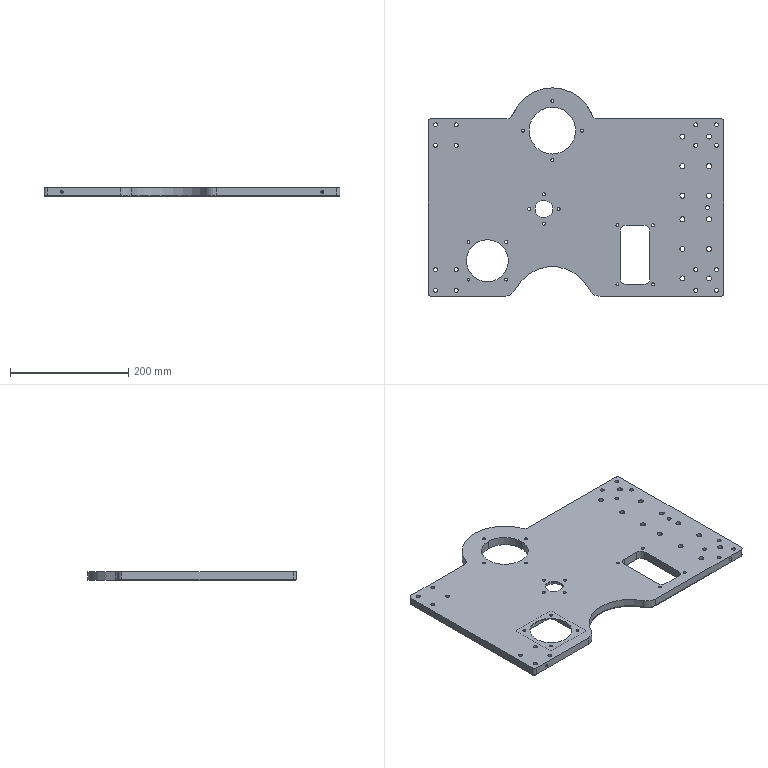NC program | Mastercam | posted with a generic post
Lines 4161 to 5460 of 11903, first 1119 of 1300 lines:
N1940 T6 M6
N1950 G0 G90 G17 G54 X237.5 Y-111.32 A0. S6000 M3
N1960 G43 H6 Z50. M8
N1970 Z1.3
N1980 G1 Z.3 F600.
N1990 G3 X235.07 Y-113.75 Z.175 I0. J-2.43 F3000.
N2000 X237.5 Y-116.18 Z.05 I2.43 J0.
N2010 X239.93 Y-113.75 Z-.075 I0. J2.43
N2020 X237.5 Y-111.32 Z-.2 I-2.43 J0.
N2030 X235.07 Y-113.75 Z-.325 I0. J-2.43
N2040 X237.5 Y-116.18 Z-.45 I2.43 J0.
N2050 X239.93 Y-113.75 Z-.575 I0. J2.43
N2060 X237.5 Y-111.32 Z-.7 I-2.43 J0.
N2070 X235.07 Y-113.75 Z-.825 I0. J-2.43
N2080 X237.5 Y-116.18 Z-.95 I2.43 J0.
N2090 X239.93 Y-113.75 Z-1.075 I0. J2.43
N2100 X237.5 Y-111.32 Z-1.2 I-2.43 J0.
N2110 X235.07 Y-113.75 Z-1.325 I0. J-2.43
N2120 X237.5 Y-116.18 Z-1.45 I2.43 J0.
N2130 X239.93 Y-113.75 Z-1.575 I0. J2.43
N2140 X237.5 Y-111.32 Z-1.7 I-2.43 J0.
N2150 X235.07 Y-113.75 Z-1.825 I0. J-2.43
N2160 X237.5 Y-116.18 Z-1.95 I2.43 J0.
N2170 X239.93 Y-113.75 Z-2.075 I0. J2.43
N2180 X237.5 Y-111.32 Z-2.2 I-2.43 J0.
N2190 X235.07 Y-113.75 Z-2.325 I0. J-2.43
N2200 X237.5 Y-116.18 Z-2.45 I2.43 J0.
N2210 X239.93 Y-113.75 Z-2.575 I0. J2.43
N2220 X237.5 Y-111.32 Z-2.7 I-2.43 J0.
N2230 X235.07 Y-113.75 Z-2.825 I0. J-2.43
N2240 X237.5 Y-116.18 Z-2.95 I2.43 J0.
N2250 X239.93 Y-113.75 Z-3.075 I0. J2.43
N2260 X237.5 Y-111.32 Z-3.2 I-2.43 J0.
N2270 X235.07 Y-113.75 Z-3.325 I0. J-2.43
N2280 X237.5 Y-116.18 Z-3.45 I2.43 J0.
N2290 X239.93 Y-113.75 Z-3.575 I0. J2.43
N2300 X237.5 Y-111.32 Z-3.7 I-2.43 J0.
N2310 X235.07 Y-113.75 Z-3.825 I0. J-2.43
N2320 X237.5 Y-116.18 Z-3.95 I2.43 J0.
N2330 X239.93 Y-113.75 Z-4.075 I0. J2.43
N2340 X237.5 Y-111.32 Z-4.2 I-2.43 J0.
N2350 X235.07 Y-113.75 Z-4.325 I0. J-2.43
N2360 X237.5 Y-116.18 Z-4.45 I2.43 J0.
N2370 X239.93 Y-113.75 Z-4.575 I0. J2.43
N2380 X237.5 Y-111.32 Z-4.7 I-2.43 J0.
N2390 X235.07 Y-113.75 Z-4.825 I0. J-2.43
N2400 X237.5 Y-116.18 Z-4.95 I2.43 J0.
N2410 X239.93 Y-113.75 Z-5.075 I0. J2.43
N2420 X237.5 Y-111.32 Z-5.2 I-2.43 J0.
N2430 X235.07 Y-113.75 Z-5.325 I0. J-2.43
N2440 X237.5 Y-116.18 Z-5.45 I2.43 J0.
N2450 X239.93 Y-113.75 Z-5.575 I0. J2.43
N2460 X237.5 Y-111.32 Z-5.7 I-2.43 J0.
N2470 X235.07 Y-113.75 Z-5.825 I0. J-2.43
N2480 X237.5 Y-116.18 Z-5.95 I2.43 J0.
N2490 X239.93 Y-113.75 Z-6.075 I0. J2.43
N2500 X237.5 Y-111.32 Z-6.2 I-2.43 J0.
N2510 X235.07 Y-113.75 Z-6.325 I0. J-2.43
N2520 X237.5 Y-116.18 Z-6.45 I2.43 J0.
N2530 X239.93 Y-113.75 Z-6.575 I0. J2.43
N2540 X237.5 Y-111.32 Z-6.7 I-2.43 J0.
N2550 X236.072 Y-111.784 Z-6.75 I0. J-2.43
N2560 X235.07 Y-113.75 I1.428 J-1.966
N2570 X237.5 Y-116.18 I2.43 J0.
N2580 X239.93 Y-113.75 I0. J2.43
N2590 X237.5 Y-111.32 I-2.43 J0.
N2600 X235.7 Y-112.117 I0. J-2.43
N2610 G0 Z50.
N2620 X202.5 Y-111.32
N2630 Z1.3
N2640 G1 Z.3 F600.
N2650 G3 X200.07 Y-113.75 Z.175 I0. J-2.43 F3000.
N2660 X202.5 Y-116.18 Z.05 I2.43 J0.
N2670 X204.93 Y-113.75 Z-.075 I0. J2.43
N2680 X202.5 Y-111.32 Z-.2 I-2.43 J0.
N2690 X200.07 Y-113.75 Z-.325 I0. J-2.43
N2700 X202.5 Y-116.18 Z-.45 I2.43 J0.
N2710 X204.93 Y-113.75 Z-.575 I0. J2.43
N2720 X202.5 Y-111.32 Z-.7 I-2.43 J0.
N2730 X200.07 Y-113.75 Z-.825 I0. J-2.43
N2740 X202.5 Y-116.18 Z-.95 I2.43 J0.
N2750 X204.93 Y-113.75 Z-1.075 I0. J2.43
N2760 X202.5 Y-111.32 Z-1.2 I-2.43 J0.
N2770 X200.07 Y-113.75 Z-1.325 I0. J-2.43
N2780 X202.5 Y-116.18 Z-1.45 I2.43 J0.
N2790 X204.93 Y-113.75 Z-1.575 I0. J2.43
N2800 X202.5 Y-111.32 Z-1.7 I-2.43 J0.
N2810 X200.07 Y-113.75 Z-1.825 I0. J-2.43
N2820 X202.5 Y-116.18 Z-1.95 I2.43 J0.
N2830 X204.93 Y-113.75 Z-2.075 I0. J2.43
N2840 X202.5 Y-111.32 Z-2.2 I-2.43 J0.
N2850 X200.07 Y-113.75 Z-2.325 I0. J-2.43
N2860 X202.5 Y-116.18 Z-2.45 I2.43 J0.
N2870 X204.93 Y-113.75 Z-2.575 I0. J2.43
N2880 X202.5 Y-111.32 Z-2.7 I-2.43 J0.
N2890 X200.07 Y-113.75 Z-2.825 I0. J-2.43
N2900 X202.5 Y-116.18 Z-2.95 I2.43 J0.
N2910 X204.93 Y-113.75 Z-3.075 I0. J2.43
N2920 X202.5 Y-111.32 Z-3.2 I-2.43 J0.
N2930 X200.07 Y-113.75 Z-3.325 I0. J-2.43
N2940 X202.5 Y-116.18 Z-3.45 I2.43 J0.
N2950 X204.93 Y-113.75 Z-3.575 I0. J2.43
N2960 X202.5 Y-111.32 Z-3.7 I-2.43 J0.
N2970 X200.07 Y-113.75 Z-3.825 I0. J-2.43
N2980 X202.5 Y-116.18 Z-3.95 I2.43 J0.
N2990 X204.93 Y-113.75 Z-4.075 I0. J2.43
N3000 X202.5 Y-111.32 Z-4.2 I-2.43 J0.
N3010 X200.07 Y-113.75 Z-4.325 I0. J-2.43
N3020 X202.5 Y-116.18 Z-4.45 I2.43 J0.
N3030 X204.93 Y-113.75 Z-4.575 I0. J2.43
N3040 X202.5 Y-111.32 Z-4.7 I-2.43 J0.
N3050 X200.07 Y-113.75 Z-4.825 I0. J-2.43
N3060 X202.5 Y-116.18 Z-4.95 I2.43 J0.
N3070 X204.93 Y-113.75 Z-5.075 I0. J2.43
N3080 X202.5 Y-111.32 Z-5.2 I-2.43 J0.
N3090 X200.07 Y-113.75 Z-5.325 I0. J-2.43
N3100 X202.5 Y-116.18 Z-5.45 I2.43 J0.
N3110 X204.93 Y-113.75 Z-5.575 I0. J2.43
N3120 X202.5 Y-111.32 Z-5.7 I-2.43 J0.
N3130 X200.07 Y-113.75 Z-5.825 I0. J-2.43
N3140 X202.5 Y-116.18 Z-5.95 I2.43 J0.
N3150 X204.93 Y-113.75 Z-6.075 I0. J2.43
N3160 X202.5 Y-111.32 Z-6.2 I-2.43 J0.
N3170 X200.07 Y-113.75 Z-6.325 I0. J-2.43
N3180 X202.5 Y-116.18 Z-6.45 I2.43 J0.
N3190 X204.93 Y-113.75 Z-6.575 I0. J2.43
N3200 X202.5 Y-111.32 Z-6.7 I-2.43 J0.
N3210 X201.072 Y-111.784 Z-6.75 I0. J-2.43
N3220 X200.07 Y-113.75 I1.428 J-1.966
N3230 X202.5 Y-116.18 I2.43 J0.
N3240 X204.93 Y-113.75 I0. J2.43
N3250 X202.5 Y-111.32 I-2.43 J0.
N3260 X200.7 Y-112.117 I0. J-2.43
N3270 G0 Z50.
N3280 X202.5 Y-76.32
N3290 Z1.3
N3300 G1 Z.3 F600.
N3310 G3 X200.07 Y-78.75 Z.175 I0. J-2.43 F3000.
N3320 X202.5 Y-81.18 Z.05 I2.43 J0.
N3330 X204.93 Y-78.75 Z-.075 I0. J2.43
N3340 X202.5 Y-76.32 Z-.2 I-2.43 J0.
N3350 X200.07 Y-78.75 Z-.325 I0. J-2.43
N3360 X202.5 Y-81.18 Z-.45 I2.43 J0.
N3370 X204.93 Y-78.75 Z-.575 I0. J2.43
N3380 X202.5 Y-76.32 Z-.7 I-2.43 J0.
N3390 X200.07 Y-78.75 Z-.825 I0. J-2.43
N3400 X202.5 Y-81.18 Z-.95 I2.43 J0.
N3410 X204.93 Y-78.75 Z-1.075 I0. J2.43
N3420 X202.5 Y-76.32 Z-1.2 I-2.43 J0.
N3430 X200.07 Y-78.75 Z-1.325 I0. J-2.43
N3440 X202.5 Y-81.18 Z-1.45 I2.43 J0.
N3450 X204.93 Y-78.75 Z-1.575 I0. J2.43
N3460 X202.5 Y-76.32 Z-1.7 I-2.43 J0.
N3470 X200.07 Y-78.75 Z-1.825 I0. J-2.43
N3480 X202.5 Y-81.18 Z-1.95 I2.43 J0.
N3490 X204.93 Y-78.75 Z-2.075 I0. J2.43
N3500 X202.5 Y-76.32 Z-2.2 I-2.43 J0.
N3510 X200.07 Y-78.75 Z-2.325 I0. J-2.43
N3520 X202.5 Y-81.18 Z-2.45 I2.43 J0.
N3530 X204.93 Y-78.75 Z-2.575 I0. J2.43
N3540 X202.5 Y-76.32 Z-2.7 I-2.43 J0.
N3550 X200.07 Y-78.75 Z-2.825 I0. J-2.43
N3560 X202.5 Y-81.18 Z-2.95 I2.43 J0.
N3570 X204.93 Y-78.75 Z-3.075 I0. J2.43
N3580 X202.5 Y-76.32 Z-3.2 I-2.43 J0.
N3590 X200.07 Y-78.75 Z-3.325 I0. J-2.43
N3600 X202.5 Y-81.18 Z-3.45 I2.43 J0.
N3610 X204.93 Y-78.75 Z-3.575 I0. J2.43
N3620 X202.5 Y-76.32 Z-3.7 I-2.43 J0.
N3630 X200.07 Y-78.75 Z-3.825 I0. J-2.43
N3640 X202.5 Y-81.18 Z-3.95 I2.43 J0.
N3650 X204.93 Y-78.75 Z-4.075 I0. J2.43
N3660 X202.5 Y-76.32 Z-4.2 I-2.43 J0.
N3670 X200.07 Y-78.75 Z-4.325 I0. J-2.43
N3680 X202.5 Y-81.18 Z-4.45 I2.43 J0.
N3690 X204.93 Y-78.75 Z-4.575 I0. J2.43
N3700 X202.5 Y-76.32 Z-4.7 I-2.43 J0.
N3710 X200.07 Y-78.75 Z-4.825 I0. J-2.43
N3720 X202.5 Y-81.18 Z-4.95 I2.43 J0.
N3730 X204.93 Y-78.75 Z-5.075 I0. J2.43
N3740 X202.5 Y-76.32 Z-5.2 I-2.43 J0.
N3750 X200.07 Y-78.75 Z-5.325 I0. J-2.43
N3760 X202.5 Y-81.18 Z-5.45 I2.43 J0.
N3770 X204.93 Y-78.75 Z-5.575 I0. J2.43
N3780 X202.5 Y-76.32 Z-5.7 I-2.43 J0.
N3790 X200.07 Y-78.75 Z-5.825 I0. J-2.43
N3800 X202.5 Y-81.18 Z-5.95 I2.43 J0.
N3810 X204.93 Y-78.75 Z-6.075 I0. J2.43
N3820 X202.5 Y-76.32 Z-6.2 I-2.43 J0.
N3830 X200.07 Y-78.75 Z-6.325 I0. J-2.43
N3840 X202.5 Y-81.18 Z-6.45 I2.43 J0.
N3850 X204.93 Y-78.75 Z-6.575 I0. J2.43
N3860 X202.5 Y-76.32 Z-6.7 I-2.43 J0.
N3870 X201.072 Y-76.784 Z-6.75 I0. J-2.43
N3880 X200.07 Y-78.75 I1.428 J-1.966
N3890 X202.5 Y-81.18 I2.43 J0.
N3900 X204.93 Y-78.75 I0. J2.43
N3910 X202.5 Y-76.32 I-2.43 J0.
N3920 X200.7 Y-77.117 I0. J-2.43
N3930 G0 Z50.
N3940 X237.5 Y-76.32
N3950 Z1.3
N3960 G1 Z.3 F600.
N3970 G3 X235.07 Y-78.75 Z.175 I0. J-2.43 F3000.
N3980 X237.5 Y-81.18 Z.05 I2.43 J0.
N3990 X239.93 Y-78.75 Z-.075 I0. J2.43
N4000 X237.5 Y-76.32 Z-.2 I-2.43 J0.
N4010 X235.07 Y-78.75 Z-.325 I0. J-2.43
N4020 X237.5 Y-81.18 Z-.45 I2.43 J0.
N4030 X239.93 Y-78.75 Z-.575 I0. J2.43
N4040 X237.5 Y-76.32 Z-.7 I-2.43 J0.
N4050 X235.07 Y-78.75 Z-.825 I0. J-2.43
N4060 X237.5 Y-81.18 Z-.95 I2.43 J0.
N4070 X239.93 Y-78.75 Z-1.075 I0. J2.43
N4080 X237.5 Y-76.32 Z-1.2 I-2.43 J0.
N4090 X235.07 Y-78.75 Z-1.325 I0. J-2.43
N4100 X237.5 Y-81.18 Z-1.45 I2.43 J0.
N4110 X239.93 Y-78.75 Z-1.575 I0. J2.43
N4120 X237.5 Y-76.32 Z-1.7 I-2.43 J0.
N4130 X235.07 Y-78.75 Z-1.825 I0. J-2.43
N4140 X237.5 Y-81.18 Z-1.95 I2.43 J0.
N4150 X239.93 Y-78.75 Z-2.075 I0. J2.43
N4160 X237.5 Y-76.32 Z-2.2 I-2.43 J0.
N4170 X235.07 Y-78.75 Z-2.325 I0. J-2.43
N4180 X237.5 Y-81.18 Z-2.45 I2.43 J0.
N4190 X239.93 Y-78.75 Z-2.575 I0. J2.43
N4200 X237.5 Y-76.32 Z-2.7 I-2.43 J0.
N4210 X235.07 Y-78.75 Z-2.825 I0. J-2.43
N4220 X237.5 Y-81.18 Z-2.95 I2.43 J0.
N4230 X239.93 Y-78.75 Z-3.075 I0. J2.43
N4240 X237.5 Y-76.32 Z-3.2 I-2.43 J0.
N4250 X235.07 Y-78.75 Z-3.325 I0. J-2.43
N4260 X237.5 Y-81.18 Z-3.45 I2.43 J0.
N4270 X239.93 Y-78.75 Z-3.575 I0. J2.43
N4280 X237.5 Y-76.32 Z-3.7 I-2.43 J0.
N4290 X235.07 Y-78.75 Z-3.825 I0. J-2.43
N4300 X237.5 Y-81.18 Z-3.95 I2.43 J0.
N4310 X239.93 Y-78.75 Z-4.075 I0. J2.43
N4320 X237.5 Y-76.32 Z-4.2 I-2.43 J0.
N4330 X235.07 Y-78.75 Z-4.325 I0. J-2.43
N4340 X237.5 Y-81.18 Z-4.45 I2.43 J0.
N4350 X239.93 Y-78.75 Z-4.575 I0. J2.43
N4360 X237.5 Y-76.32 Z-4.7 I-2.43 J0.
N4370 X235.07 Y-78.75 Z-4.825 I0. J-2.43
N4380 X237.5 Y-81.18 Z-4.95 I2.43 J0.
N4390 X239.93 Y-78.75 Z-5.075 I0. J2.43
N4400 X237.5 Y-76.32 Z-5.2 I-2.43 J0.
N4410 X235.07 Y-78.75 Z-5.325 I0. J-2.43
N4420 X237.5 Y-81.18 Z-5.45 I2.43 J0.
N4430 X239.93 Y-78.75 Z-5.575 I0. J2.43
N4440 X237.5 Y-76.32 Z-5.7 I-2.43 J0.
N4450 X235.07 Y-78.75 Z-5.825 I0. J-2.43
N4460 X237.5 Y-81.18 Z-5.95 I2.43 J0.
N4470 X239.93 Y-78.75 Z-6.075 I0. J2.43
N4480 X237.5 Y-76.32 Z-6.2 I-2.43 J0.
N4490 X235.07 Y-78.75 Z-6.325 I0. J-2.43
N4500 X237.5 Y-81.18 Z-6.45 I2.43 J0.
N4510 X239.93 Y-78.75 Z-6.575 I0. J2.43
N4520 X237.5 Y-76.32 Z-6.7 I-2.43 J0.
N4530 X236.072 Y-76.784 Z-6.75 I0. J-2.43
N4540 X235.07 Y-78.75 I1.428 J-1.966
N4550 X237.5 Y-81.18 I2.43 J0.
N4560 X239.93 Y-78.75 I0. J2.43
N4570 X237.5 Y-76.32 I-2.43 J0.
N4580 X235.7 Y-77.117 I0. J-2.43
N4590 G0 Z50.
N4600 X237.5 Y133.68
N4610 Z1.3
N4620 G1 Z.3 F600.
N4630 G3 X235.07 Y131.25 Z.175 I0. J-2.43 F3000.
N4640 X237.5 Y128.82 Z.05 I2.43 J0.
N4650 X239.93 Y131.25 Z-.075 I0. J2.43
N4660 X237.5 Y133.68 Z-.2 I-2.43 J0.
N4670 X235.07 Y131.25 Z-.325 I0. J-2.43
N4680 X237.5 Y128.82 Z-.45 I2.43 J0.
N4690 X239.93 Y131.25 Z-.575 I0. J2.43
N4700 X237.5 Y133.68 Z-.7 I-2.43 J0.
N4710 X235.07 Y131.25 Z-.825 I0. J-2.43
N4720 X237.5 Y128.82 Z-.95 I2.43 J0.
N4730 X239.93 Y131.25 Z-1.075 I0. J2.43
N4740 X237.5 Y133.68 Z-1.2 I-2.43 J0.
N4750 X235.07 Y131.25 Z-1.325 I0. J-2.43
N4760 X237.5 Y128.82 Z-1.45 I2.43 J0.
N4770 X239.93 Y131.25 Z-1.575 I0. J2.43
N4780 X237.5 Y133.68 Z-1.7 I-2.43 J0.
N4790 X235.07 Y131.25 Z-1.825 I0. J-2.43
N4800 X237.5 Y128.82 Z-1.95 I2.43 J0.
N4810 X239.93 Y131.25 Z-2.075 I0. J2.43
N4820 X237.5 Y133.68 Z-2.2 I-2.43 J0.
N4830 X235.07 Y131.25 Z-2.325 I0. J-2.43
N4840 X237.5 Y128.82 Z-2.45 I2.43 J0.
N4850 X239.93 Y131.25 Z-2.575 I0. J2.43
N4860 X237.5 Y133.68 Z-2.7 I-2.43 J0.
N4870 X235.07 Y131.25 Z-2.825 I0. J-2.43
N4880 X237.5 Y128.82 Z-2.95 I2.43 J0.
N4890 X239.93 Y131.25 Z-3.075 I0. J2.43
N4900 X237.5 Y133.68 Z-3.2 I-2.43 J0.
N4910 X235.07 Y131.25 Z-3.325 I0. J-2.43
N4920 X237.5 Y128.82 Z-3.45 I2.43 J0.
N4930 X239.93 Y131.25 Z-3.575 I0. J2.43
N4940 X237.5 Y133.68 Z-3.7 I-2.43 J0.
N4950 X235.07 Y131.25 Z-3.825 I0. J-2.43
N4960 X237.5 Y128.82 Z-3.95 I2.43 J0.
N4970 X239.93 Y131.25 Z-4.075 I0. J2.43
N4980 X237.5 Y133.68 Z-4.2 I-2.43 J0.
N4990 X235.07 Y131.25 Z-4.325 I0. J-2.43
N5000 X237.5 Y128.82 Z-4.45 I2.43 J0.
N5010 X239.93 Y131.25 Z-4.575 I0. J2.43
N5020 X237.5 Y133.68 Z-4.7 I-2.43 J0.
N5030 X235.07 Y131.25 Z-4.825 I0. J-2.43
N5040 X237.5 Y128.82 Z-4.95 I2.43 J0.
N5050 X239.93 Y131.25 Z-5.075 I0. J2.43
N5060 X237.5 Y133.68 Z-5.2 I-2.43 J0.
N5070 X235.07 Y131.25 Z-5.325 I0. J-2.43
N5080 X237.5 Y128.82 Z-5.45 I2.43 J0.
N5090 X239.93 Y131.25 Z-5.575 I0. J2.43
N5100 X237.5 Y133.68 Z-5.7 I-2.43 J0.
N5110 X235.07 Y131.25 Z-5.825 I0. J-2.43
N5120 X237.5 Y128.82 Z-5.95 I2.43 J0.
N5130 X239.93 Y131.25 Z-6.075 I0. J2.43
N5140 X237.5 Y133.68 Z-6.2 I-2.43 J0.
N5150 X235.07 Y131.25 Z-6.325 I0. J-2.43
N5160 X237.5 Y128.82 Z-6.45 I2.43 J0.
N5170 X239.93 Y131.25 Z-6.575 I0. J2.43
N5180 X237.5 Y133.68 Z-6.7 I-2.43 J0.
N5190 X236.072 Y133.216 Z-6.75 I0. J-2.43
N5200 X235.07 Y131.25 I1.428 J-1.966
N5210 X237.5 Y128.82 I2.43 J0.
N5220 X239.93 Y131.25 I0. J2.43
N5230 X237.5 Y133.68 I-2.43 J0.
N5240 X235.7 Y132.883 I0. J-2.43
N5250 G0 Z50.
N5260 X202.5 Y133.68
N5270 Z1.3
N5280 G1 Z.3 F600.
N5290 G3 X200.07 Y131.25 Z.175 I0. J-2.43 F3000.
N5300 X202.5 Y128.82 Z.05 I2.43 J0.
N5310 X204.93 Y131.25 Z-.075 I0. J2.43
N5320 X202.5 Y133.68 Z-.2 I-2.43 J0.
N5330 X200.07 Y131.25 Z-.325 I0. J-2.43
N5340 X202.5 Y128.82 Z-.45 I2.43 J0.
N5350 X204.93 Y131.25 Z-.575 I0. J2.43
N5360 X202.5 Y133.68 Z-.7 I-2.43 J0.
N5370 X200.07 Y131.25 Z-.825 I0. J-2.43
N5380 X202.5 Y128.82 Z-.95 I2.43 J0.
N5390 X204.93 Y131.25 Z-1.075 I0. J2.43
N5400 X202.5 Y133.68 Z-1.2 I-2.43 J0.
N5410 X200.07 Y131.25 Z-1.325 I0. J-2.43
N5420 X202.5 Y128.82 Z-1.45 I2.43 J0.
N5430 X204.93 Y131.25 Z-1.575 I0. J2.43
N5440 X202.5 Y133.68 Z-1.7 I-2.43 J0.
N5450 X200.07 Y131.25 Z-1.825 I0. J-2.43
N5460 X202.5 Y128.82 Z-1.95 I2.43 J0.
N5470 X204.93 Y131.25 Z-2.075 I0. J2.43
N5480 X202.5 Y133.68 Z-2.2 I-2.43 J0.
N5490 X200.07 Y131.25 Z-2.325 I0. J-2.43
N5500 X202.5 Y128.82 Z-2.45 I2.43 J0.
N5510 X204.93 Y131.25 Z-2.575 I0. J2.43
N5520 X202.5 Y133.68 Z-2.7 I-2.43 J0.
N5530 X200.07 Y131.25 Z-2.825 I0. J-2.43
N5540 X202.5 Y128.82 Z-2.95 I2.43 J0.
N5550 X204.93 Y131.25 Z-3.075 I0. J2.43
N5560 X202.5 Y133.68 Z-3.2 I-2.43 J0.
N5570 X200.07 Y131.25 Z-3.325 I0. J-2.43
N5580 X202.5 Y128.82 Z-3.45 I2.43 J0.
N5590 X204.93 Y131.25 Z-3.575 I0. J2.43
N5600 X202.5 Y133.68 Z-3.7 I-2.43 J0.
N5610 X200.07 Y131.25 Z-3.825 I0. J-2.43
N5620 X202.5 Y128.82 Z-3.95 I2.43 J0.
N5630 X204.93 Y131.25 Z-4.075 I0. J2.43
N5640 X202.5 Y133.68 Z-4.2 I-2.43 J0.
N5650 X200.07 Y131.25 Z-4.325 I0. J-2.43
N5660 X202.5 Y128.82 Z-4.45 I2.43 J0.
N5670 X204.93 Y131.25 Z-4.575 I0. J2.43
N5680 X202.5 Y133.68 Z-4.7 I-2.43 J0.
N5690 X200.07 Y131.25 Z-4.825 I0. J-2.43
N5700 X202.5 Y128.82 Z-4.95 I2.43 J0.
N5710 X204.93 Y131.25 Z-5.075 I0. J2.43
N5720 X202.5 Y133.68 Z-5.2 I-2.43 J0.
N5730 X200.07 Y131.25 Z-5.325 I0. J-2.43
N5740 X202.5 Y128.82 Z-5.45 I2.43 J0.
N5750 X204.93 Y131.25 Z-5.575 I0. J2.43
N5760 X202.5 Y133.68 Z-5.7 I-2.43 J0.
N5770 X200.07 Y131.25 Z-5.825 I0. J-2.43
N5780 X202.5 Y128.82 Z-5.95 I2.43 J0.
N5790 X204.93 Y131.25 Z-6.075 I0. J2.43
N5800 X202.5 Y133.68 Z-6.2 I-2.43 J0.
N5810 X200.07 Y131.25 Z-6.325 I0. J-2.43
N5820 X202.5 Y128.82 Z-6.45 I2.43 J0.
N5830 X204.93 Y131.25 Z-6.575 I0. J2.43
N5840 X202.5 Y133.68 Z-6.7 I-2.43 J0.
N5850 X201.072 Y133.216 Z-6.75 I0. J-2.43
N5860 X200.07 Y131.25 I1.428 J-1.966
N5870 X202.5 Y128.82 I2.43 J0.
N5880 X204.93 Y131.25 I0. J2.43
N5890 X202.5 Y133.68 I-2.43 J0.
N5900 X200.7 Y132.883 I0. J-2.43
N5910 G0 Z50.
N5920 X-202.5 Y133.68
N5930 Z1.3
N5940 G1 Z.3 F600.
N5950 G3 X-204.93 Y131.25 Z.175 I0. J-2.43 F3000.
N5960 X-202.5 Y128.82 Z.05 I2.43 J0.
N5970 X-200.07 Y131.25 Z-.075 I0. J2.43
N5980 X-202.5 Y133.68 Z-.2 I-2.43 J0.
N5990 X-204.93 Y131.25 Z-.325 I0. J-2.43
N6000 X-202.5 Y128.82 Z-.45 I2.43 J0.
N6010 X-200.07 Y131.25 Z-.575 I0. J2.43
N6020 X-202.5 Y133.68 Z-.7 I-2.43 J0.
N6030 X-204.93 Y131.25 Z-.825 I0. J-2.43
N6040 X-202.5 Y128.82 Z-.95 I2.43 J0.
N6050 X-200.07 Y131.25 Z-1.075 I0. J2.43
N6060 X-202.5 Y133.68 Z-1.2 I-2.43 J0.
N6070 X-204.93 Y131.25 Z-1.325 I0. J-2.43
N6080 X-202.5 Y128.82 Z-1.45 I2.43 J0.
N6090 X-200.07 Y131.25 Z-1.575 I0. J2.43
N6100 X-202.5 Y133.68 Z-1.7 I-2.43 J0.
N6110 X-204.93 Y131.25 Z-1.825 I0. J-2.43
N6120 X-202.5 Y128.82 Z-1.95 I2.43 J0.
N6130 X-200.07 Y131.25 Z-2.075 I0. J2.43
N6140 X-202.5 Y133.68 Z-2.2 I-2.43 J0.
N6150 X-204.93 Y131.25 Z-2.325 I0. J-2.43
N6160 X-202.5 Y128.82 Z-2.45 I2.43 J0.
N6170 X-200.07 Y131.25 Z-2.575 I0. J2.43
N6180 X-202.5 Y133.68 Z-2.7 I-2.43 J0.
N6190 X-204.93 Y131.25 Z-2.825 I0. J-2.43
N6200 X-202.5 Y128.82 Z-2.95 I2.43 J0.
N6210 X-200.07 Y131.25 Z-3.075 I0. J2.43
N6220 X-202.5 Y133.68 Z-3.2 I-2.43 J0.
N6230 X-204.93 Y131.25 Z-3.325 I0. J-2.43
N6240 X-202.5 Y128.82 Z-3.45 I2.43 J0.
N6250 X-200.07 Y131.25 Z-3.575 I0. J2.43
N6260 X-202.5 Y133.68 Z-3.7 I-2.43 J0.
N6270 X-204.93 Y131.25 Z-3.825 I0. J-2.43
N6280 X-202.5 Y128.82 Z-3.95 I2.43 J0.
N6290 X-200.07 Y131.25 Z-4.075 I0. J2.43
N6300 X-202.5 Y133.68 Z-4.2 I-2.43 J0.
N6310 X-204.93 Y131.25 Z-4.325 I0. J-2.43
N6320 X-202.5 Y128.82 Z-4.45 I2.43 J0.
N6330 X-200.07 Y131.25 Z-4.575 I0. J2.43
N6340 X-202.5 Y133.68 Z-4.7 I-2.43 J0.
N6350 X-204.93 Y131.25 Z-4.825 I0. J-2.43
N6360 X-202.5 Y128.82 Z-4.95 I2.43 J0.
N6370 X-200.07 Y131.25 Z-5.075 I0. J2.43
N6380 X-202.5 Y133.68 Z-5.2 I-2.43 J0.
N6390 X-204.93 Y131.25 Z-5.325 I0. J-2.43
N6400 X-202.5 Y128.82 Z-5.45 I2.43 J0.
N6410 X-200.07 Y131.25 Z-5.575 I0. J2.43
N6420 X-202.5 Y133.68 Z-5.7 I-2.43 J0.
N6430 X-204.93 Y131.25 Z-5.825 I0. J-2.43
N6440 X-202.5 Y128.82 Z-5.95 I2.43 J0.
N6450 X-200.07 Y131.25 Z-6.075 I0. J2.43
N6460 X-202.5 Y133.68 Z-6.2 I-2.43 J0.
N6470 X-204.93 Y131.25 Z-6.325 I0. J-2.43
N6480 X-202.5 Y128.82 Z-6.45 I2.43 J0.
N6490 X-200.07 Y131.25 Z-6.575 I0. J2.43
N6500 X-202.5 Y133.68 Z-6.7 I-2.43 J0.
N6510 X-203.928 Y133.216 Z-6.75 I0. J-2.43
N6520 X-204.93 Y131.25 I1.428 J-1.966
N6530 X-202.5 Y128.82 I2.43 J0.
N6540 X-200.07 Y131.25 I0. J2.43
N6550 X-202.5 Y133.68 I-2.43 J0.
N6560 X-204.3 Y132.883 I0. J-2.43
N6570 G0 Z50.
N6580 X-237.5 Y133.68
N6590 Z1.3
N6600 G1 Z.3 F600.
N6610 G3 X-239.93 Y131.25 Z.175 I0. J-2.43 F3000.
N6620 X-237.5 Y128.82 Z.05 I2.43 J0.
N6630 X-235.07 Y131.25 Z-.075 I0. J2.43
N6640 X-237.5 Y133.68 Z-.2 I-2.43 J0.
N6650 X-239.93 Y131.25 Z-.325 I0. J-2.43
N6660 X-237.5 Y128.82 Z-.45 I2.43 J0.
N6670 X-235.07 Y131.25 Z-.575 I0. J2.43
N6680 X-237.5 Y133.68 Z-.7 I-2.43 J0.
N6690 X-239.93 Y131.25 Z-.825 I0. J-2.43
N6700 X-237.5 Y128.82 Z-.95 I2.43 J0.
N6710 X-235.07 Y131.25 Z-1.075 I0. J2.43
N6720 X-237.5 Y133.68 Z-1.2 I-2.43 J0.
N6730 X-239.93 Y131.25 Z-1.325 I0. J-2.43
N6740 X-237.5 Y128.82 Z-1.45 I2.43 J0.
N6750 X-235.07 Y131.25 Z-1.575 I0. J2.43
N6760 X-237.5 Y133.68 Z-1.7 I-2.43 J0.
N6770 X-239.93 Y131.25 Z-1.825 I0. J-2.43
N6780 X-237.5 Y128.82 Z-1.95 I2.43 J0.
N6790 X-235.07 Y131.25 Z-2.075 I0. J2.43
N6800 X-237.5 Y133.68 Z-2.2 I-2.43 J0.
N6810 X-239.93 Y131.25 Z-2.325 I0. J-2.43
N6820 X-237.5 Y128.82 Z-2.45 I2.43 J0.
N6830 X-235.07 Y131.25 Z-2.575 I0. J2.43
N6840 X-237.5 Y133.68 Z-2.7 I-2.43 J0.
N6850 X-239.93 Y131.25 Z-2.825 I0. J-2.43
N6860 X-237.5 Y128.82 Z-2.95 I2.43 J0.
N6870 X-235.07 Y131.25 Z-3.075 I0. J2.43
N6880 X-237.5 Y133.68 Z-3.2 I-2.43 J0.
N6890 X-239.93 Y131.25 Z-3.325 I0. J-2.43
N6900 X-237.5 Y128.82 Z-3.45 I2.43 J0.
N6910 X-235.07 Y131.25 Z-3.575 I0. J2.43
N6920 X-237.5 Y133.68 Z-3.7 I-2.43 J0.
N6930 X-239.93 Y131.25 Z-3.825 I0. J-2.43
N6940 X-237.5 Y128.82 Z-3.95 I2.43 J0.
N6950 X-235.07 Y131.25 Z-4.075 I0. J2.43
N6960 X-237.5 Y133.68 Z-4.2 I-2.43 J0.
N6970 X-239.93 Y131.25 Z-4.325 I0. J-2.43
N6980 X-237.5 Y128.82 Z-4.45 I2.43 J0.
N6990 X-235.07 Y131.25 Z-4.575 I0. J2.43
N7000 X-237.5 Y133.68 Z-4.7 I-2.43 J0.
N7010 X-239.93 Y131.25 Z-4.825 I0. J-2.43
N7020 X-237.5 Y128.82 Z-4.95 I2.43 J0.
N7030 X-235.07 Y131.25 Z-5.075 I0. J2.43
N7040 X-237.5 Y133.68 Z-5.2 I-2.43 J0.
N7050 X-239.93 Y131.25 Z-5.325 I0. J-2.43
N7060 X-237.5 Y128.82 Z-5.45 I2.43 J0.
N7070 X-235.07 Y131.25 Z-5.575 I0. J2.43
N7080 X-237.5 Y133.68 Z-5.7 I-2.43 J0.
N7090 X-239.93 Y131.25 Z-5.825 I0. J-2.43
N7100 X-237.5 Y128.82 Z-5.95 I2.43 J0.
N7110 X-235.07 Y131.25 Z-6.075 I0. J2.43
N7120 X-237.5 Y133.68 Z-6.2 I-2.43 J0.
N7130 X-239.93 Y131.25 Z-6.325 I0. J-2.43
N7140 X-237.5 Y128.82 Z-6.45 I2.43 J0.
N7150 X-235.07 Y131.25 Z-6.575 I0. J2.43
N7160 X-237.5 Y133.68 Z-6.7 I-2.43 J0.
N7170 X-238.928 Y133.216 Z-6.75 I0. J-2.43
N7180 X-239.93 Y131.25 I1.428 J-1.966
N7190 X-237.5 Y128.82 I2.43 J0.
N7200 X-235.07 Y131.25 I0. J2.43
N7210 X-237.5 Y133.68 I-2.43 J0.
N7220 X-239.3 Y132.883 I0. J-2.43
N7230 G0 Z50.
N7240 X-237.5 Y-76.32
N7250 Z1.3
N7260 G1 Z.3 F600.
N7270 G3 X-239.93 Y-78.75 Z.175 I0. J-2.43 F3000.
N7280 X-237.5 Y-81.18 Z.05 I2.43 J0.
N7290 X-235.07 Y-78.75 Z-.075 I0. J2.43
N7300 X-237.5 Y-76.32 Z-.2 I-2.43 J0.
N7310 X-239.93 Y-78.75 Z-.325 I0. J-2.43
N7320 X-237.5 Y-81.18 Z-.45 I2.43 J0.
N7330 X-235.07 Y-78.75 Z-.575 I0. J2.43
N7340 X-237.5 Y-76.32 Z-.7 I-2.43 J0.
N7350 X-239.93 Y-78.75 Z-.825 I0. J-2.43
N7360 X-237.5 Y-81.18 Z-.95 I2.43 J0.
N7370 X-235.07 Y-78.75 Z-1.075 I0. J2.43
N7380 X-237.5 Y-76.32 Z-1.2 I-2.43 J0.
N7390 X-239.93 Y-78.75 Z-1.325 I0. J-2.43
N7400 X-237.5 Y-81.18 Z-1.45 I2.43 J0.
N7410 X-235.07 Y-78.75 Z-1.575 I0. J2.43
N7420 X-237.5 Y-76.32 Z-1.7 I-2.43 J0.
N7430 X-239.93 Y-78.75 Z-1.825 I0. J-2.43
N7440 X-237.5 Y-81.18 Z-1.95 I2.43 J0.
N7450 X-235.07 Y-78.75 Z-2.075 I0. J2.43
N7460 X-237.5 Y-76.32 Z-2.2 I-2.43 J0.
N7470 X-239.93 Y-78.75 Z-2.325 I0. J-2.43
N7480 X-237.5 Y-81.18 Z-2.45 I2.43 J0.
N7490 X-235.07 Y-78.75 Z-2.575 I0. J2.43
N7500 X-237.5 Y-76.32 Z-2.7 I-2.43 J0.
N7510 X-239.93 Y-78.75 Z-2.825 I0. J-2.43
N7520 X-237.5 Y-81.18 Z-2.95 I2.43 J0.
N7530 X-235.07 Y-78.75 Z-3.075 I0. J2.43
N7540 X-237.5 Y-76.32 Z-3.2 I-2.43 J0.
N7550 X-239.93 Y-78.75 Z-3.325 I0. J-2.43
N7560 X-237.5 Y-81.18 Z-3.45 I2.43 J0.
N7570 X-235.07 Y-78.75 Z-3.575 I0. J2.43
N7580 X-237.5 Y-76.32 Z-3.7 I-2.43 J0.
N7590 X-239.93 Y-78.75 Z-3.825 I0. J-2.43
N7600 X-237.5 Y-81.18 Z-3.95 I2.43 J0.
N7610 X-235.07 Y-78.75 Z-4.075 I0. J2.43
N7620 X-237.5 Y-76.32 Z-4.2 I-2.43 J0.
N7630 X-239.93 Y-78.75 Z-4.325 I0. J-2.43
N7640 X-237.5 Y-81.18 Z-4.45 I2.43 J0.
N7650 X-235.07 Y-78.75 Z-4.575 I0. J2.43
N7660 X-237.5 Y-76.32 Z-4.7 I-2.43 J0.
N7670 X-239.93 Y-78.75 Z-4.825 I0. J-2.43
N7680 X-237.5 Y-81.18 Z-4.95 I2.43 J0.
N7690 X-235.07 Y-78.75 Z-5.075 I0. J2.43
N7700 X-237.5 Y-76.32 Z-5.2 I-2.43 J0.
N7710 X-239.93 Y-78.75 Z-5.325 I0. J-2.43
N7720 X-237.5 Y-81.18 Z-5.45 I2.43 J0.
N7730 X-235.07 Y-78.75 Z-5.575 I0. J2.43
N7740 X-237.5 Y-76.32 Z-5.7 I-2.43 J0.
N7750 X-239.93 Y-78.75 Z-5.825 I0. J-2.43
N7760 X-237.5 Y-81.18 Z-5.95 I2.43 J0.
N7770 X-235.07 Y-78.75 Z-6.075 I0. J2.43
N7780 X-237.5 Y-76.32 Z-6.2 I-2.43 J0.
N7790 X-239.93 Y-78.75 Z-6.325 I0. J-2.43
N7800 X-237.5 Y-81.18 Z-6.45 I2.43 J0.
N7810 X-235.07 Y-78.75 Z-6.575 I0. J2.43
N7820 X-237.5 Y-76.32 Z-6.7 I-2.43 J0.
N7830 X-238.928 Y-76.784 Z-6.75 I0. J-2.43
N7840 X-239.93 Y-78.75 I1.428 J-1.966
N7850 X-237.5 Y-81.18 I2.43 J0.
N7860 X-235.07 Y-78.75 I0. J2.43
N7870 X-237.5 Y-76.32 I-2.43 J0.
N7880 X-239.3 Y-77.117 I0. J-2.43
N7890 G0 Z50.
N7900 X-202.5 Y-76.32
N7910 Z1.3
N7920 G1 Z.3 F600.
N7930 G3 X-204.93 Y-78.75 Z.175 I0. J-2.43 F3000.
N7940 X-202.5 Y-81.18 Z.05 I2.43 J0.
N7950 X-200.07 Y-78.75 Z-.075 I0. J2.43
N7960 X-202.5 Y-76.32 Z-.2 I-2.43 J0.
N7970 X-204.93 Y-78.75 Z-.325 I0. J-2.43
N7980 X-202.5 Y-81.18 Z-.45 I2.43 J0.
N7990 X-200.07 Y-78.75 Z-.575 I0. J2.43
N8000 X-202.5 Y-76.32 Z-.7 I-2.43 J0.
N8010 X-204.93 Y-78.75 Z-.825 I0. J-2.43
N8020 X-202.5 Y-81.18 Z-.95 I2.43 J0.
N8030 X-200.07 Y-78.75 Z-1.075 I0. J2.43
N8040 X-202.5 Y-76.32 Z-1.2 I-2.43 J0.
N8050 X-204.93 Y-78.75 Z-1.325 I0. J-2.43
N8060 X-202.5 Y-81.18 Z-1.45 I2.43 J0.
N8070 X-200.07 Y-78.75 Z-1.575 I0. J2.43
N8080 X-202.5 Y-76.32 Z-1.7 I-2.43 J0.
N8090 X-204.93 Y-78.75 Z-1.825 I0. J-2.43
N8100 X-202.5 Y-81.18 Z-1.95 I2.43 J0.
N8110 X-200.07 Y-78.75 Z-2.075 I0. J2.43
N8120 X-202.5 Y-76.32 Z-2.2 I-2.43 J0.
N8130 X-204.93 Y-78.75 Z-2.325 I0. J-2.43
N8140 X-202.5 Y-81.18 Z-2.45 I2.43 J0.
N8150 X-200.07 Y-78.75 Z-2.575 I0. J2.43
N8160 X-202.5 Y-76.32 Z-2.7 I-2.43 J0.
N8170 X-204.93 Y-78.75 Z-2.825 I0. J-2.43
N8180 X-202.5 Y-81.18 Z-2.95 I2.43 J0.
N8190 X-200.07 Y-78.75 Z-3.075 I0. J2.43
N8200 X-202.5 Y-76.32 Z-3.2 I-2.43 J0.
N8210 X-204.93 Y-78.75 Z-3.325 I0. J-2.43
N8220 X-202.5 Y-81.18 Z-3.45 I2.43 J0.
N8230 X-200.07 Y-78.75 Z-3.575 I0. J2.43
N8240 X-202.5 Y-76.32 Z-3.7 I-2.43 J0.
N8250 X-204.93 Y-78.75 Z-3.825 I0. J-2.43
N8260 X-202.5 Y-81.18 Z-3.95 I2.43 J0.
N8270 X-200.07 Y-78.75 Z-4.075 I0. J2.43
N8280 X-202.5 Y-76.32 Z-4.2 I-2.43 J0.
N8290 X-204.93 Y-78.75 Z-4.325 I0. J-2.43
N8300 X-202.5 Y-81.18 Z-4.45 I2.43 J0.
N8310 X-200.07 Y-78.75 Z-4.575 I0. J2.43
N8320 X-202.5 Y-76.32 Z-4.7 I-2.43 J0.
N8330 X-204.93 Y-78.75 Z-4.825 I0. J-2.43
N8340 X-202.5 Y-81.18 Z-4.95 I2.43 J0.
N8350 X-200.07 Y-78.75 Z-5.075 I0. J2.43
N8360 X-202.5 Y-76.32 Z-5.2 I-2.43 J0.
N8370 X-204.93 Y-78.75 Z-5.325 I0. J-2.43
N8380 X-202.5 Y-81.18 Z-5.45 I2.43 J0.
N8390 X-200.07 Y-78.75 Z-5.575 I0. J2.43
N8400 X-202.5 Y-76.32 Z-5.7 I-2.43 J0.
N8410 X-204.93 Y-78.75 Z-5.825 I0. J-2.43
N8420 X-202.5 Y-81.18 Z-5.95 I2.43 J0.
N8430 X-200.07 Y-78.75 Z-6.075 I0. J2.43
N8440 X-202.5 Y-76.32 Z-6.2 I-2.43 J0.
N8450 X-204.93 Y-78.75 Z-6.325 I0. J-2.43
N8460 X-202.5 Y-81.18 Z-6.45 I2.43 J0.
N8470 X-200.07 Y-78.75 Z-6.575 I0. J2.43
N8480 X-202.5 Y-76.32 Z-6.7 I-2.43 J0.
N8490 X-203.928 Y-76.784 Z-6.75 I0. J-2.43
N8500 X-204.93 Y-78.75 I1.428 J-1.966
N8510 X-202.5 Y-81.18 I2.43 J0.
N8520 X-200.07 Y-78.75 I0. J2.43
N8530 X-202.5 Y-76.32 I-2.43 J0.
N8540 X-204.3 Y-77.117 I0. J-2.43
N8550 G0 Z50.
N8560 X-202.5 Y-111.32
N8570 Z1.3
N8580 G1 Z.3 F600.
N8590 G3 X-204.93 Y-113.75 Z.175 I0. J-2.43 F3000.
N8600 X-202.5 Y-116.18 Z.05 I2.43 J0.
N8610 X-200.07 Y-113.75 Z-.075 I0. J2.43
N8620 X-202.5 Y-111.32 Z-.2 I-2.43 J0.
N8630 X-204.93 Y-113.75 Z-.325 I0. J-2.43
N8640 X-202.5 Y-116.18 Z-.45 I2.43 J0.
N8650 X-200.07 Y-113.75 Z-.575 I0. J2.43
N8660 X-202.5 Y-111.32 Z-.7 I-2.43 J0.
N8670 X-204.93 Y-113.75 Z-.825 I0. J-2.43
N8680 X-202.5 Y-116.18 Z-.95 I2.43 J0.
N8690 X-200.07 Y-113.75 Z-1.075 I0. J2.43
N8700 X-202.5 Y-111.32 Z-1.2 I-2.43 J0.
N8710 X-204.93 Y-113.75 Z-1.325 I0. J-2.43
N8720 X-202.5 Y-116.18 Z-1.45 I2.43 J0.
N8730 X-200.07 Y-113.75 Z-1.575 I0. J2.43
N8740 X-202.5 Y-111.32 Z-1.7 I-2.43 J0.
N8750 X-204.93 Y-113.75 Z-1.825 I0. J-2.43
N8760 X-202.5 Y-116.18 Z-1.95 I2.43 J0.
N8770 X-200.07 Y-113.75 Z-2.075 I0. J2.43
N8780 X-202.5 Y-111.32 Z-2.2 I-2.43 J0.
N8790 X-204.93 Y-113.75 Z-2.325 I0. J-2.43
N8800 X-202.5 Y-116.18 Z-2.45 I2.43 J0.
N8810 X-200.07 Y-113.75 Z-2.575 I0. J2.43
N8820 X-202.5 Y-111.32 Z-2.7 I-2.43 J0.
N8830 X-204.93 Y-113.75 Z-2.825 I0. J-2.43
N8840 X-202.5 Y-116.18 Z-2.95 I2.43 J0.
N8850 X-200.07 Y-113.75 Z-3.075 I0. J2.43
N8860 X-202.5 Y-111.32 Z-3.2 I-2.43 J0.
N8870 X-204.93 Y-113.75 Z-3.325 I0. J-2.43
N8880 X-202.5 Y-116.18 Z-3.45 I2.43 J0.
N8890 X-200.07 Y-113.75 Z-3.575 I0. J2.43
N8900 X-202.5 Y-111.32 Z-3.7 I-2.43 J0.
N8910 X-204.93 Y-113.75 Z-3.825 I0. J-2.43
N8920 X-202.5 Y-116.18 Z-3.95 I2.43 J0.
N8930 X-200.07 Y-113.75 Z-4.075 I0. J2.43
N8940 X-202.5 Y-111.32 Z-4.2 I-2.43 J0.
N8950 X-204.93 Y-113.75 Z-4.325 I0. J-2.43
N8960 X-202.5 Y-116.18 Z-4.45 I2.43 J0.
N8970 X-200.07 Y-113.75 Z-4.575 I0. J2.43
N8980 X-202.5 Y-111.32 Z-4.7 I-2.43 J0.
N8990 X-204.93 Y-113.75 Z-4.825 I0. J-2.43
N9000 X-202.5 Y-116.18 Z-4.95 I2.43 J0.
N9010 X-200.07 Y-113.75 Z-5.075 I0. J2.43
N9020 X-202.5 Y-111.32 Z-5.2 I-2.43 J0.
N9030 X-204.93 Y-113.75 Z-5.325 I0. J-2.43
N9040 X-202.5 Y-116.18 Z-5.45 I2.43 J0.
N9050 X-200.07 Y-113.75 Z-5.575 I0. J2.43
N9060 X-202.5 Y-111.32 Z-5.7 I-2.43 J0.
N9070 X-204.93 Y-113.75 Z-5.825 I0. J-2.43
N9080 X-202.5 Y-116.18 Z-5.95 I2.43 J0.
N9090 X-200.07 Y-113.75 Z-6.075 I0. J2.43
N9100 X-202.5 Y-111.32 Z-6.2 I-2.43 J0.
N9110 X-204.93 Y-113.75 Z-6.325 I0. J-2.43
N9120 X-202.5 Y-116.18 Z-6.45 I2.43 J0.
N9130 X-200.07 Y-113.75 Z-6.575 I0. J2.43
N9140 X-202.5 Y-111.32 Z-6.7 I-2.43 J0.
N9150 X-203.928 Y-111.784 Z-6.75 I0. J-2.43
N9160 X-204.93 Y-113.75 I1.428 J-1.966
N9170 X-202.5 Y-116.18 I2.43 J0.
N9180 X-200.07 Y-113.75 I0. J2.43
N9190 X-202.5 Y-111.32 I-2.43 J0.
N9200 X-204.3 Y-112.117 I0. J-2.43
N9210 G0 Z50.
N9220 X-237.5 Y-111.32
N9230 Z1.3
N9240 G1 Z.3 F600.
N9250 G3 X-239.93 Y-113.75 Z.175 I0. J-2.43 F3000.
N9260 X-237.5 Y-116.18 Z.05 I2.43 J0.
N9270 X-235.07 Y-113.75 Z-.075 I0. J2.43
N9280 X-237.5 Y-111.32 Z-.2 I-2.43 J0.
N9290 X-239.93 Y-113.75 Z-.325 I0. J-2.43
N9300 X-237.5 Y-116.18 Z-.45 I2.43 J0.
N9310 X-235.07 Y-113.75 Z-.575 I0. J2.43
N9320 X-237.5 Y-111.32 Z-.7 I-2.43 J0.
N9330 X-239.93 Y-113.75 Z-.825 I0. J-2.43
N9340 X-237.5 Y-116.18 Z-.95 I2.43 J0.
N9350 X-235.07 Y-113.75 Z-1.075 I0. J2.43
N9360 X-237.5 Y-111.32 Z-1.2 I-2.43 J0.
N9370 X-239.93 Y-113.75 Z-1.325 I0. J-2.43
N9380 X-237.5 Y-116.18 Z-1.45 I2.43 J0.
N9390 X-235.07 Y-113.75 Z-1.575 I0. J2.43
N9400 X-237.5 Y-111.32 Z-1.7 I-2.43 J0.
N9410 X-239.93 Y-113.75 Z-1.825 I0. J-2.43
N9420 X-237.5 Y-116.18 Z-1.95 I2.43 J0.
N9430 X-235.07 Y-113.75 Z-2.075 I0. J2.43
N9440 X-237.5 Y-111.32 Z-2.2 I-2.43 J0.
N9450 X-239.93 Y-113.75 Z-2.325 I0. J-2.43
N9460 X-237.5 Y-116.18 Z-2.45 I2.43 J0.
N9470 X-235.07 Y-113.75 Z-2.575 I0. J2.43
N9480 X-237.5 Y-111.32 Z-2.7 I-2.43 J0.
N9490 X-239.93 Y-113.75 Z-2.825 I0. J-2.43
N9500 X-237.5 Y-116.18 Z-2.95 I2.43 J0.
N9510 X-235.07 Y-113.75 Z-3.075 I0. J2.43
N9520 X-237.5 Y-111.32 Z-3.2 I-2.43 J0.
N9530 X-239.93 Y-113.75 Z-3.325 I0. J-2.43
N9540 X-237.5 Y-116.18 Z-3.45 I2.43 J0.
N9550 X-235.07 Y-113.75 Z-3.575 I0. J2.43
N9560 X-237.5 Y-111.32 Z-3.7 I-2.43 J0.
N9570 X-239.93 Y-113.75 Z-3.825 I0. J-2.43
N9580 X-237.5 Y-116.18 Z-3.95 I2.43 J0.
N9590 X-235.07 Y-113.75 Z-4.075 I0. J2.43
N9600 X-237.5 Y-111.32 Z-4.2 I-2.43 J0.
N9610 X-239.93 Y-113.75 Z-4.325 I0. J-2.43
N9620 X-237.5 Y-116.18 Z-4.45 I2.43 J0.
N9630 X-235.07 Y-113.75 Z-4.575 I0. J2.43
N9640 X-237.5 Y-111.32 Z-4.7 I-2.43 J0.
N9650 X-239.93 Y-113.75 Z-4.825 I0. J-2.43
N9660 X-237.5 Y-116.18 Z-4.95 I2.43 J0.
N9670 X-235.07 Y-113.75 Z-5.075 I0. J2.43
N9680 X-237.5 Y-111.32 Z-5.2 I-2.43 J0.
N9690 X-239.93 Y-113.75 Z-5.325 I0. J-2.43
N9700 X-237.5 Y-116.18 Z-5.45 I2.43 J0.
N9710 X-235.07 Y-113.75 Z-5.575 I0. J2.43
N9720 X-237.5 Y-111.32 Z-5.7 I-2.43 J0.
N9730 X-239.93 Y-113.75 Z-5.825 I0. J-2.43
N9740 X-237.5 Y-116.18 Z-5.95 I2.43 J0.
N9750 X-235.07 Y-113.75 Z-6.075 I0. J2.43
N9760 X-237.5 Y-111.32 Z-6.2 I-2.43 J0.
N9770 X-239.93 Y-113.75 Z-6.325 I0. J-2.43
N9780 X-237.5 Y-116.18 Z-6.45 I2.43 J0.
N9790 X-235.07 Y-113.75 Z-6.575 I0. J2.43
N9800 X-237.5 Y-111.32 Z-6.7 I-2.43 J0.
N9810 X-238.928 Y-111.784 Z-6.75 I0. J-2.43
N9820 X-239.93 Y-113.75 I1.428 J-1.966
N9830 X-237.5 Y-116.18 I2.43 J0.
N9840 X-235.07 Y-113.75 I0. J2.43
N9850 X-237.5 Y-111.32 I-2.43 J0.
N9860 X-239.3 Y-112.117 I0. J-2.43
N9870 G0 Z50.
N9880 X238.1 Y-112.43
N9890 Z1.3
N9900 G1 Z.3 F600.
N9910 Y-111.83 F1000.
N9920 G3 X237.5 Y-111.23 I-.6 J0.
N9930 X234.98 Y-113.75 Z-.95 I0. J-2.52
N9940 X237.5 Y-116.27 Z-2.2 I2.52 J0.
N9950 X240.02 Y-113.75 Z-3.45 I0. J2.52
N9960 X237.5 Y-111.23 Z-4.7 I-2.52 J0.
N9970 X234.98 Y-113.75 Z-5.95 I0. J-2.52
N9980 X236.286 Y-115.958 Z-6.8 I2.52 J0.
N9990 X237.5 Y-116.27 I1.214 J2.208
N100 X240.02 Y-113.75 I0. J2.52
N110 X237.5 Y-111.23 I-2.52 J0.
N120 X234.98 Y-113.75 I0. J-2.52
N130 X236.745 Y-116.154 I2.52 J0.
N140 X236.925 Y-116.182 I.18 J.572
N150 X237.497 Y-115.762 I0. J.6
N160 G1 X237.677 Y-115.189
N170 G0 Z50.
N180 X203.1 Y-112.43
N190 Z1.3
N200 G1 Z.3 F600.
N210 Y-111.83 F1000.
N220 G3 X202.5 Y-111.23 I-.6 J0.
N230 X199.98 Y-113.75 Z-.95 I0. J-2.52
N240 X202.5 Y-116.27 Z-2.2 I2.52 J0.
N250 X205.02 Y-113.75 Z-3.45 I0. J2.52
N260 X202.5 Y-111.23 Z-4.7 I-2.52 J0.
N270 X199.98 Y-113.75 Z-5.95 I0. J-2.52
N280 X201.286 Y-115.958 Z-6.8 I2.52 J0.
N290 X202.5 Y-116.27 I1.214 J2.208
N300 X205.02 Y-113.75 I0. J2.52
N310 X202.5 Y-111.23 I-2.52 J0.
N320 X199.98 Y-113.75 I0. J-2.52
N330 X201.745 Y-116.154 I2.52 J0.
N340 X201.925 Y-116.182 I.18 J.572
N350 X202.497 Y-115.762 I0. J.6
N360 G1 X202.677 Y-115.189
N370 G0 Z50.
N380 X203.1 Y-77.43
N390 Z1.3
N400 G1 Z.3 F600.
N410 Y-76.83 F1000.
N420 G3 X202.5 Y-76.23 I-.6 J0.
N430 X199.98 Y-78.75 Z-.95 I0. J-2.52
N440 X202.5 Y-81.27 Z-2.2 I2.52 J0.
N450 X205.02 Y-78.75 Z-3.45 I0. J2.52
N460 X202.5 Y-76.23 Z-4.7 I-2.52 J0.
N470 X199.98 Y-78.75 Z-5.95 I0. J-2.52
N480 X201.286 Y-80.958 Z-6.8 I2.52 J0.
N490 X202.5 Y-81.27 I1.214 J2.208
N500 X205.02 Y-78.75 I0. J2.52
N510 X202.5 Y-76.23 I-2.52 J0.
N520 X199.98 Y-78.75 I0. J-2.52
N530 X201.745 Y-81.154 I2.52 J0.
N540 X201.925 Y-81.182 I.18 J.572
N550 X202.497 Y-80.762 I0. J.6
N560 G1 X202.677 Y-80.189
N570 G0 Z50.
N580 X238.1 Y-77.43
N590 Z1.3
N600 G1 Z.3 F600.
N610 Y-76.83 F1000.
N620 G3 X237.5 Y-76.23 I-.6 J0.
N630 X234.98 Y-78.75 Z-.95 I0. J-2.52
N640 X237.5 Y-81.27 Z-2.2 I2.52 J0.
N650 X240.02 Y-78.75 Z-3.45 I0. J2.52
N660 X237.5 Y-76.23 Z-4.7 I-2.52 J0.
N670 X234.98 Y-78.75 Z-5.95 I0. J-2.52
N680 X236.286 Y-80.958 Z-6.8 I2.52 J0.
N690 X237.5 Y-81.27 I1.214 J2.208
N700 X240.02 Y-78.75 I0. J2.52
N710 X237.5 Y-76.23 I-2.52 J0.
N720 X234.98 Y-78.75 I0. J-2.52
N730 X236.745 Y-81.154 I2.52 J0.
N740 X236.925 Y-81.182 I.18 J.572
N750 X237.497 Y-80.762 I0. J.6
N760 G1 X237.677 Y-80.189
N770 G0 Z50.
N780 X238.1 Y132.57
N790 Z1.3
N800 G1 Z.3 F600.
N810 Y133.17 F1000.
N820 G3 X237.5 Y133.77 I-.6 J0.
N830 X234.98 Y131.25 Z-.95 I0. J-2.52
N840 X237.5 Y128.73 Z-2.2 I2.52 J0.
N850 X240.02 Y131.25 Z-3.45 I0. J2.52
N860 X237.5 Y133.77 Z-4.7 I-2.52 J0.
N870 X234.98 Y131.25 Z-5.95 I0. J-2.52
N880 X236.286 Y129.042 Z-6.8 I2.52 J0.
N890 X237.5 Y128.73 I1.214 J2.208
N900 X240.02 Y131.25 I0. J2.52
N910 X237.5 Y133.77 I-2.52 J0.
N920 X234.98 Y131.25 I0. J-2.52
N930 X236.745 Y128.846 I2.52 J0.
N940 X236.925 Y128.818 I.18 J.572
N950 X237.497 Y129.238 I0. J.6
N960 G1 X237.677 Y129.811
N970 G0 Z50.
N980 X203.1 Y132.57
N990 Z1.3
N1000 G1 Z.3 F600.
N1010 Y133.17 F1000.
N1020 G3 X202.5 Y133.77 I-.6 J0.
N1030 X199.98 Y131.25 Z-.95 I0. J-2.52
N1040 X202.5 Y128.73 Z-2.2 I2.52 J0.
N1050 X205.02 Y131.25 Z-3.45 I0. J2.52
N1060 X202.5 Y133.77 Z-4.7 I-2.52 J0.
N1070 X199.98 Y131.25 Z-5.95 I0. J-2.52
N1080 X201.286 Y129.042 Z-6.8 I2.52 J0.
N1090 X202.5 Y128.73 I1.214 J2.208
N1100 X205.02 Y131.25 I0. J2.52
N1110 X202.5 Y133.77 I-2.52 J0.
N1120 X199.98 Y131.25 I0. J-2.52
N1130 X201.745 Y128.846 I2.52 J0.
N1140 X201.925 Y128.818 I.18 J.572
N1150 X202.497 Y129.238 I0. J.6
N1160 G1 X202.677 Y129.811
N1170 G0 Z50.
N1180 X-201.9 Y132.57
N1190 Z1.3
N1200 G1 Z.3 F600.
N1210 Y133.17 F1000.
N1220 G3 X-202.5 Y133.77 I-.6 J0.
N1230 X-205.02 Y131.25 Z-.95 I0. J-2.52
N1240 X-202.5 Y128.73 Z-2.2 I2.52 J0.
N1250 X-199.98 Y131.25 Z-3.45 I0. J2.52
N1260 X-202.5 Y133.77 Z-4.7 I-2.52 J0.
N1270 X-205.02 Y131.25 Z-5.95 I0. J-2.52
N1280 X-203.714 Y129.042 Z-6.8 I2.52 J0.
N1290 X-202.5 Y128.73 I1.214 J2.208
N1300 X-199.98 Y131.25 I0. J2.52
N1310 X-202.5 Y133.77 I-2.52 J0.
N1320 X-205.02 Y131.25 I0. J-2.52
N1330 X-203.255 Y128.846 I2.52 J0.
N1340 X-203.075 Y128.818 I.18 J.572
N1350 X-202.503 Y129.238 I0. J.6
N1360 G1 X-202.323 Y129.811
N1370 G0 Z50.
N1380 X-236.9 Y132.57
N1390 Z1.3
N1400 G1 Z.3 F600.
N1410 Y133.17 F1000.
N1420 G3 X-237.5 Y133.77 I-.6 J0.
N1430 X-240.02 Y131.25 Z-.95 I0. J-2.52
N1440 X-237.5 Y128.73 Z-2.2 I2.52 J0.
N1450 X-234.98 Y131.25 Z-3.45 I0. J2.52
N1460 X-237.5 Y133.77 Z-4.7 I-2.52 J0.
N1470 X-240.02 Y131.25 Z-5.95 I0. J-2.52
N1480 X-238.714 Y129.042 Z-6.8 I2.52 J0.
N1490 X-237.5 Y128.73 I1.214 J2.208
N1500 X-234.98 Y131.25 I0. J2.52
N1510 X-237.5 Y133.77 I-2.52 J0.
N1520 X-240.02 Y131.25 I0. J-2.52
N1530 X-238.255 Y128.846 I2.52 J0.
N1540 X-238.075 Y128.818 I.18 J.572
N1550 X-237.503 Y129.238 I0. J.6
N1560 G1 X-237.323 Y129.811
N1570 G0 Z50.
N1580 X-236.9 Y-77.43
N1590 Z1.3
N1600 G1 Z.3 F600.
N1610 Y-76.83 F1000.
N1620 G3 X-237.5 Y-76.23 I-.6 J0.
N1630 X-240.02 Y-78.75 Z-.95 I0. J-2.52
N1640 X-237.5 Y-81.27 Z-2.2 I2.52 J0.
N1650 X-234.98 Y-78.75 Z-3.45 I0. J2.52
N1660 X-237.5 Y-76.23 Z-4.7 I-2.52 J0.
N1670 X-240.02 Y-78.75 Z-5.95 I0. J-2.52
N1680 X-238.714 Y-80.958 Z-6.8 I2.52 J0.
N1690 X-237.5 Y-81.27 I1.214 J2.208
N1700 X-234.98 Y-78.75 I0. J2.52
N1710 X-237.5 Y-76.23 I-2.52 J0.
N1720 X-240.02 Y-78.75 I0. J-2.52
N1730 X-238.255 Y-81.154 I2.52 J0.
N1740 X-238.075 Y-81.182 I.18 J.572
N1750 X-237.503 Y-80.762 I0. J.6
N1760 G1 X-237.323 Y-80.189
N1770 G0 Z50.
N1780 X-201.9 Y-77.43
N1790 Z1.3
N1800 G1 Z.3 F600.
N1810 Y-76.83 F1000.
N1820 G3 X-202.5 Y-76.23 I-.6 J0.
N1830 X-205.02 Y-78.75 Z-.95 I0. J-2.52
N1840 X-202.5 Y-81.27 Z-2.2 I2.52 J0.
N1850 X-199.98 Y-78.75 Z-3.45 I0. J2.52
N1860 X-202.5 Y-76.23 Z-4.7 I-2.52 J0.
N1870 X-205.02 Y-78.75 Z-5.95 I0. J-2.52
N1880 X-203.714 Y-80.958 Z-6.8 I2.52 J0.
N1890 X-202.5 Y-81.27 I1.214 J2.208
N1900 X-199.98 Y-78.75 I0. J2.52
N1910 X-202.5 Y-76.23 I-2.52 J0.
N1920 X-205.02 Y-78.75 I0. J-2.52
N1930 X-203.255 Y-81.154 I2.52 J0.
N1940 X-203.075 Y-81.182 I.18 J.572
N1950 X-202.503 Y-80.762 I0. J.6
N1960 G1 X-202.323 Y-80.189
N1970 G0 Z50.
N1980 X-201.9 Y-112.43
N1990 Z1.3
N2000 G1 Z.3 F600.
N2010 Y-111.83 F1000.
N2020 G3 X-202.5 Y-111.23 I-.6 J0.
N2030 X-205.02 Y-113.75 Z-.95 I0. J-2.52
N2040 X-202.5 Y-116.27 Z-2.2 I2.52 J0.
N2050 X-199.98 Y-113.75 Z-3.45 I0. J2.52
N2060 X-202.5 Y-111.23 Z-4.7 I-2.52 J0.
N2070 X-205.02 Y-113.75 Z-5.95 I0. J-2.52
N2080 X-203.714 Y-115.958 Z-6.8 I2.52 J0.
N2090 X-202.5 Y-116.27 I1.214 J2.208
N2100 X-199.98 Y-113.75 I0. J2.52
N2110 X-202.5 Y-111.23 I-2.52 J0.
N2120 X-205.02 Y-113.75 I0. J-2.52
N2130 X-203.255 Y-116.154 I2.52 J0.
N2140 X-203.075 Y-116.182 I.18 J.572
N2150 X-202.503 Y-115.762 I0. J.6
N2160 G1 X-202.323 Y-115.189
N2170 G0 Z50.
N2180 X-236.9 Y-112.43
N2190 Z1.3
N2200 G1 Z.3 F600.
N2210 Y-111.83 F1000.
N2220 G3 X-237.5 Y-111.23 I-.6 J0.
N2230 X-240.02 Y-113.75 Z-.95 I0. J-2.52
N2240 X-237.5 Y-116.27 Z-2.2 I2.52 J0.
N2250 X-234.98 Y-113.75 Z-3.45 I0. J2.52
N2260 X-237.5 Y-111.23 Z-4.7 I-2.52 J0.
N2270 X-240.02 Y-113.75 Z-5.95 I0. J-2.52
N2280 X-238.714 Y-115.958 Z-6.8 I2.52 J0.
N2290 X-237.5 Y-116.27 I1.214 J2.208
N2300 X-234.98 Y-113.75 I0. J2.52
N2310 X-237.5 Y-111.23 I-2.52 J0.
N2320 X-240.02 Y-113.75 I0. J-2.52
N2330 X-238.255 Y-116.154 I2.52 J0.
N2340 X-238.075 Y-116.182 I.18 J.572
N2350 X-237.503 Y-115.762 I0. J.6
N2360 G1 X-237.323 Y-115.189
N2370 G0 Z50.
N2380 M5
N2390 G91 G28 Z0. M9
N2400 A0.
N2410 M01
N2420 T11 M6
N2430 G0 G90 G17 G54 X-254. Y-128.75 A0. S6500 M3
N2440 G43 H11 Z50. M8
N2450 Z2.
N2460 G1 Z-3. F600.
N2470 Y-118.75 F4000.
N2480 Y171.25
N2490 Y181.25
N2500 Z-2.821
N2510 X-253.995
N2520 Y171.25
N2530 Y-118.75
N2540 Y-128.75
N2550 Z-2.639
N2560 X-253.978
N2570 Y-118.75
N2580 Y171.25
N2590 Y181.25
N2600 Z-2.454
N2610 X-253.95
N2620 Y171.25
N2630 Y-118.75
N2640 Y-128.75
N2650 Z-2.268
N2660 X-253.909
N2670 Y-118.75
N2680 Y171.25
N2690 Y181.25
N2700 Z-2.081
N2710 X-253.856
N2720 Y171.25
N2730 Y-118.75
N2740 Y-128.75
N2750 Z-1.896
N2760 X-253.789
N2770 Y-118.75
N2780 Y171.25
N2790 Y181.25
N2800 Z-1.712
N2810 X-253.71
N2820 Y171.25
N2830 Y-118.75
N2840 Y-128.75
N2850 Z-1.533
N2860 X-253.617
N2870 Y-118.75
N2880 Y171.25
N2890 Y181.25
N2900 Z-1.358
N2910 X-253.511
N2920 Y171.25
N2930 Y-118.75
N2940 Y-128.75
N2950 Z-1.19
N2960 X-253.393
N2970 Y-118.75
N2980 Y171.25
N2990 Y181.25
N3000 Z-1.03
N3010 X-253.263
N3020 Y171.25
N3030 Y-118.75
N3040 Y-128.75
N3050 Z-.879
N3060 X-253.121
N3070 Y-118.75
N3080 Y171.25
N3090 Y181.25
N3100 Z-.737
N3110 X-252.97
N3120 Y171.25
N3130 Y-118.75
N3140 Y-128.75
N3150 Z-.607
N3160 X-252.81
N3170 Y-118.75
N3180 Y171.25
N3190 Y181.25
N3200 Z-.489
N3210 X-252.642
N3220 Y171.25